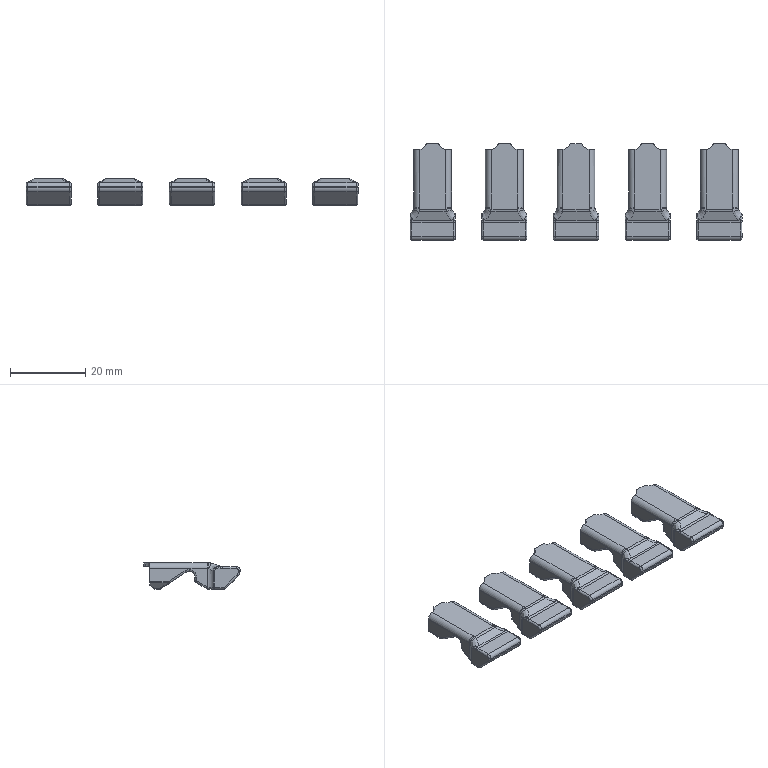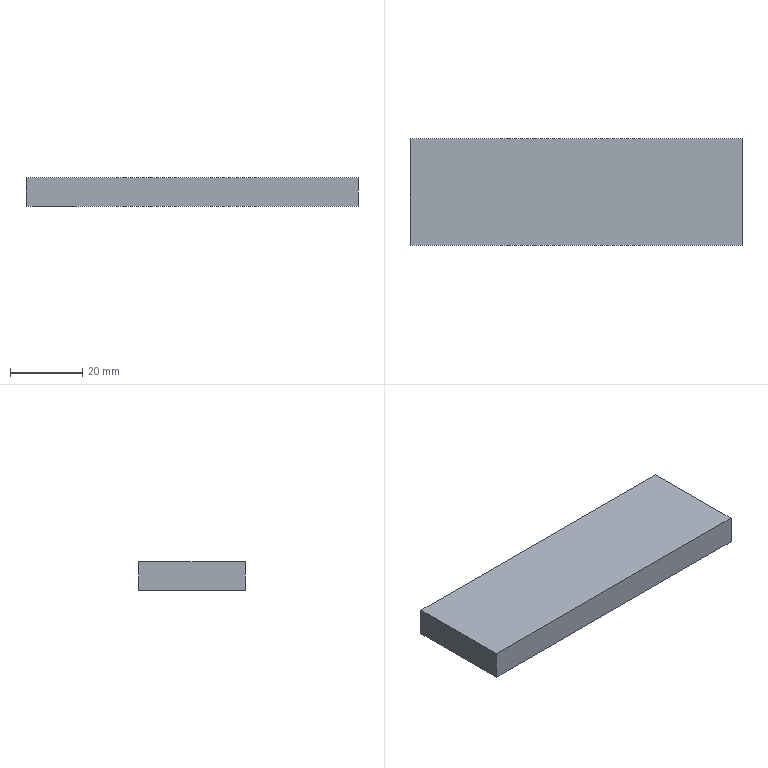CAM job | NX | 3-axis milling | part box 88 x 25.5 x 7 mm | stock box 92 x 29.5 x 8 mm
Tools:
number,name,description,diameter,corner_radius,flute_length,length,flutes
19,D80,Milling Tool-5 Parameters,80.0,0.0,50.0,75.0,2
11,D4,Milling Tool-5 Parameters,4.0,0.0,50.0,75.0,2
16,D3,Milling Tool-5 Parameters,3.0,0.0,50.0,75.0,2
17,R1.5,Milling Tool-5 Parameters,3.0,1.5,50.0,75.0,2
18,D4R0.5,Milling Tool-5 Parameters,4.0,0.5,50.0,75.0,2
Operations:
program,operation,operation_type,tool,method,geometry_group,spindle_rpm,surface_speed,feed_per_tooth,feed_cut,feed_plunge,cut_length_mm,path_length_mm,cut_time_min,machine_time_min
1AB胶,FLOOR_WALL,VolumeBased25DMillingOperation,D80,METHOD,A,6500.0,1633.0,0.1154,1500.0,100.0,184.0,238.0,0.1227,0.1281
1AB胶,ZLEVEL_PROFILE,ZLevelMilling,D4,METHOD,A,9500.0,119.0,0.1474,2800.0,1000.0,8638.176,9286.23,3.198,3.263
1AB胶,CAVITY_MILL,CavityMilling,D4,METHOD,A,9500.0,119.0,0.1316,2500.0,1000.0,16869.969,17154.883,6.784,6.812
1AB胶,FLOOR_WALL_1,VolumeBased25DMillingOperation,D4,METHOD,A,9500.0,89.0,0.0711,1350.0,100.0,161.34,367.541,0.1195,0.1401
1AB胶,CAVITY_MILL_COPY,CavityMilling,D3,METHOD,A,9500.0,89.0,0.0947,1800.0,1000.0,593.687,1102.013,0.4119,0.4627
1AB胶,FIXED_CONTOUR,SurfaceContour,R1.5,METHOD,A,9500.0,59.0,0.1316,2500.0,100.0,29566.897,30081.368,11.827,11.878
1AB胶,ZLEVEL_PROFILE_COPY,ZLevelMilling,D4,METHOD,A,9500.0,119.0,0.0632,1200.0,1000.0,1878.319,2370.85,1.591,1.64
2,FIXED_CONTOUR_COPY,SurfaceContour,D4R0.5,METHOD,B,9500.0,59.0,0.1316,2500.0,100.0,6139.681,6197.969,2.456,2.462